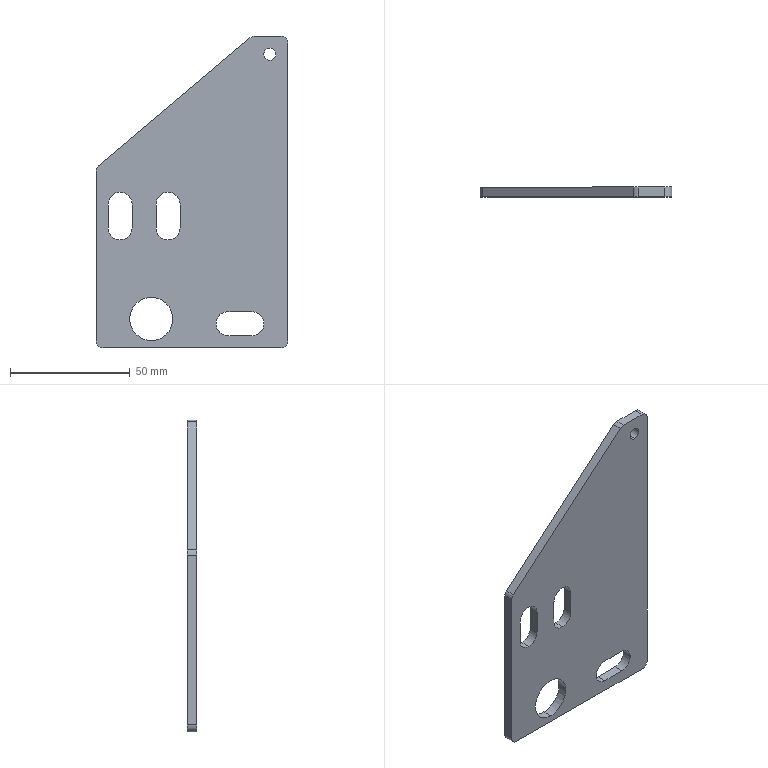Part | SolidWorks | features ExtruRefSurface 1, Extrusion 1, Fillet 1 | 1 solid | 30 faces | box 80 x 4 x 130 mm | volume 31186 mm3 | cylinder 17 | plane 13 | commonest cylinder face diameters 10 x8 6 x5 5 x2 18 x2
STEP:
#1=CARTESIAN_POINT('',(-7.5,4.,120.));
#2=VERTEX_POINT('',#1);
#3=CARTESIAN_POINT('',(-7.5,4.,125.));
#4=VERTEX_POINT('',#3);
#5=CARTESIAN_POINT('',(-7.5,4.,122.5));
#6=DIRECTION('',(0.,1.,0.));
#7=DIRECTION('',(0.,0.,1.));
#8=AXIS2_PLACEMENT_3D('',#5,#6,#7);
#9=CIRCLE('',#8,2.5);
#10=EDGE_CURVE('',#2,#4,#9,.T.);
#11=ORIENTED_EDGE('',*,*,#10,.T.);
#12=CARTESIAN_POINT('',(-7.5,0.,125.));
#13=VERTEX_POINT('',#12);
#14=CARTESIAN_POINT('',(-7.5,4.,125.));
#15=DIRECTION('',(0.,-1.,0.));
#16=VECTOR('',#15,1000.);
#17=LINE('',#14,#16);
#18=EDGE_CURVE('',#4,#13,#17,.T.);
#19=ORIENTED_EDGE('',*,*,#18,.T.);
#20=CARTESIAN_POINT('',(-7.5,0.,120.));
#21=VERTEX_POINT('',#20);
#22=CARTESIAN_POINT('',(-7.5,0.,122.5));
#23=DIRECTION('',(0.,1.,0.));
#24=DIRECTION('',(0.,0.,1.));
#25=AXIS2_PLACEMENT_3D('',#22,#23,#24);
#26=CIRCLE('',#25,2.5);
#27=EDGE_CURVE('',#21,#13,#26,.T.);
#28=ORIENTED_EDGE('',*,*,#27,.F.);
#29=CARTESIAN_POINT('',(-7.5,4.,120.));
#30=DIRECTION('',(0.,-1.,0.));
#31=VECTOR('',#30,1000.);
#32=LINE('',#29,#31);
#33=EDGE_CURVE('',#2,#21,#32,.T.);
#34=ORIENTED_EDGE('',*,*,#33,.F.);
#35=EDGE_LOOP('',(#11,#19,#28,#34));
#36=FACE_OUTER_BOUND('',#35,.T.);
#37=CARTESIAN_POINT('',(-7.5,4.,122.5));
#38=DIRECTION('',(0.,-1.,0.));
#39=DIRECTION('',(0.,0.,-1.));
#40=AXIS2_PLACEMENT_3D('',#37,#38,#39);
#41=CYLINDRICAL_SURFACE('',#40,2.5);
#42=ADVANCED_FACE('',(#36),#41,.F.);
#43=CARTESIAN_POINT('',(-45.,4.,50.));
#44=VERTEX_POINT('',#43);
#45=CARTESIAN_POINT('',(-50.,4.,45.));
#46=VERTEX_POINT('',#45);
#47=CARTESIAN_POINT('',(-50.,4.,50.));
#48=DIRECTION('',(0.,1.,0.));
#49=DIRECTION('',(0.,0.,1.));
#50=AXIS2_PLACEMENT_3D('',#47,#48,#49);
#51=CIRCLE('',#50,5.);
#52=EDGE_CURVE('',#44,#46,#51,.T.);
#53=ORIENTED_EDGE('',*,*,#52,.T.);
#54=CARTESIAN_POINT('',(-50.,0.,45.));
#55=VERTEX_POINT('',#54);
#56=CARTESIAN_POINT('',(-50.,4.,45.));
#57=DIRECTION('',(0.,-1.,0.));
#58=VECTOR('',#57,1000.);
#59=LINE('',#56,#58);
#60=EDGE_CURVE('',#46,#55,#59,.T.);
#61=ORIENTED_EDGE('',*,*,#60,.T.);
#62=CARTESIAN_POINT('',(-45.,0.,50.));
#63=VERTEX_POINT('',#62);
#64=CARTESIAN_POINT('',(-50.,0.,50.));
#65=DIRECTION('',(0.,1.,0.));
#66=DIRECTION('',(0.,0.,1.));
#67=AXIS2_PLACEMENT_3D('',#64,#65,#66);
#68=CIRCLE('',#67,5.);
#69=EDGE_CURVE('',#63,#55,#68,.T.);
#70=ORIENTED_EDGE('',*,*,#69,.F.);
#71=CARTESIAN_POINT('',(-45.,4.,50.));
#72=DIRECTION('',(0.,-1.,0.));
#73=VECTOR('',#72,1000.);
#74=LINE('',#71,#73);
#75=EDGE_CURVE('',#44,#63,#74,.T.);
#76=ORIENTED_EDGE('',*,*,#75,.F.);
#77=EDGE_LOOP('',(#53,#61,#70,#76));
#78=FACE_OUTER_BOUND('',#77,.T.);
#79=CARTESIAN_POINT('',(-50.,4.,50.));
#80=DIRECTION('',(0.,-1.,0.));
#81=DIRECTION('',(0.,0.,-1.));
#82=AXIS2_PLACEMENT_3D('',#79,#80,#81);
#83=CYLINDRICAL_SURFACE('',#82,5.);
#84=ADVANCED_FACE('',(#78),#83,.F.);
#85=CARTESIAN_POINT('',(-65.,4.,50.));
#86=VERTEX_POINT('',#85);
#87=CARTESIAN_POINT('',(-70.,4.,45.));
#88=VERTEX_POINT('',#87);
#89=CARTESIAN_POINT('',(-70.,4.,50.));
#90=DIRECTION('',(0.,1.,0.));
#91=DIRECTION('',(0.,0.,1.));
#92=AXIS2_PLACEMENT_3D('',#89,#90,#91);
#93=CIRCLE('',#92,5.);
#94=EDGE_CURVE('',#86,#88,#93,.T.);
#95=ORIENTED_EDGE('',*,*,#94,.T.);
#96=CARTESIAN_POINT('',(-70.,0.,45.));
#97=VERTEX_POINT('',#96);
#98=CARTESIAN_POINT('',(-70.,4.,45.));
#99=DIRECTION('',(0.,-1.,0.));
#100=VECTOR('',#99,1000.);
#101=LINE('',#98,#100);
#102=EDGE_CURVE('',#88,#97,#101,.T.);
#103=ORIENTED_EDGE('',*,*,#102,.T.);
#104=CARTESIAN_POINT('',(-65.,0.,50.));
#105=VERTEX_POINT('',#104);
#106=CARTESIAN_POINT('',(-70.,0.,50.));
#107=DIRECTION('',(0.,1.,0.));
#108=DIRECTION('',(0.,0.,1.));
#109=AXIS2_PLACEMENT_3D('',#106,#107,#108);
#110=CIRCLE('',#109,5.);
#111=EDGE_CURVE('',#105,#97,#110,.T.);
#112=ORIENTED_EDGE('',*,*,#111,.F.);
#113=CARTESIAN_POINT('',(-65.,4.,50.));
#114=DIRECTION('',(0.,-1.,0.));
#115=VECTOR('',#114,1000.);
#116=LINE('',#113,#115);
#117=EDGE_CURVE('',#86,#105,#116,.T.);
#118=ORIENTED_EDGE('',*,*,#117,.F.);
#119=EDGE_LOOP('',(#95,#103,#112,#118));
#120=FACE_OUTER_BOUND('',#119,.T.);
#121=CARTESIAN_POINT('',(-70.,4.,50.));
#122=DIRECTION('',(0.,-1.,0.));
#123=DIRECTION('',(0.,0.,-1.));
#124=AXIS2_PLACEMENT_3D('',#121,#122,#123);
#125=CYLINDRICAL_SURFACE('',#124,5.);
#126=ADVANCED_FACE('',(#120),#125,.F.);
#127=CARTESIAN_POINT('',(-57.,4.,3.));
#128=VERTEX_POINT('',#127);
#129=CARTESIAN_POINT('',(-57.,4.,21.));
#130=VERTEX_POINT('',#129);
#131=CARTESIAN_POINT('',(-57.,4.,12.));
#132=DIRECTION('',(0.,1.,0.));
#133=DIRECTION('',(0.,0.,1.));
#134=AXIS2_PLACEMENT_3D('',#131,#132,#133);
#135=CIRCLE('',#134,9.);
#136=EDGE_CURVE('',#128,#130,#135,.T.);
#137=ORIENTED_EDGE('',*,*,#136,.T.);
#138=CARTESIAN_POINT('',(-57.,0.,21.));
#139=VERTEX_POINT('',#138);
#140=CARTESIAN_POINT('',(-57.,4.,21.));
#141=DIRECTION('',(0.,-1.,0.));
#142=VECTOR('',#141,1000.);
#143=LINE('',#140,#142);
#144=EDGE_CURVE('',#130,#139,#143,.T.);
#145=ORIENTED_EDGE('',*,*,#144,.T.);
#146=CARTESIAN_POINT('',(-57.,0.,3.));
#147=VERTEX_POINT('',#146);
#148=CARTESIAN_POINT('',(-57.,0.,12.));
#149=DIRECTION('',(0.,1.,0.));
#150=DIRECTION('',(0.,0.,1.));
#151=AXIS2_PLACEMENT_3D('',#148,#149,#150);
#152=CIRCLE('',#151,9.);
#153=EDGE_CURVE('',#147,#139,#152,.T.);
#154=ORIENTED_EDGE('',*,*,#153,.F.);
#155=CARTESIAN_POINT('',(-57.,4.,3.));
#156=DIRECTION('',(0.,-1.,0.));
#157=VECTOR('',#156,1000.);
#158=LINE('',#155,#157);
#159=EDGE_CURVE('',#128,#147,#158,.T.);
#160=ORIENTED_EDGE('',*,*,#159,.F.);
#161=EDGE_LOOP('',(#137,#145,#154,#160));
#162=FACE_OUTER_BOUND('',#161,.T.);
#163=CARTESIAN_POINT('',(-57.,4.,12.));
#164=DIRECTION('',(0.,-1.,0.));
#165=DIRECTION('',(0.,0.,-1.));
#166=AXIS2_PLACEMENT_3D('',#163,#164,#165);
#167=CYLINDRICAL_SURFACE('',#166,9.);
#168=ADVANCED_FACE('',(#162),#167,.F.);
#169=CARTESIAN_POINT('',(-55.,4.,50.));
#170=VERTEX_POINT('',#169);
#171=CARTESIAN_POINT('',(-55.,4.,60.));
#172=VERTEX_POINT('',#171);
#173=CARTESIAN_POINT('',(-55.,4.,50.));
#174=DIRECTION('',(0.,0.,1.));
#175=VECTOR('',#174,1000.);
#176=LINE('',#173,#175);
#177=EDGE_CURVE('',#170,#172,#176,.T.);
#178=ORIENTED_EDGE('',*,*,#177,.F.);
#179=CARTESIAN_POINT('',(-50.,4.,50.));
#180=DIRECTION('',(0.,1.,0.));
#181=DIRECTION('',(0.,0.,1.));
#182=AXIS2_PLACEMENT_3D('',#179,#180,#181);
#183=CIRCLE('',#182,5.);
#184=EDGE_CURVE('',#46,#170,#183,.T.);
#185=ORIENTED_EDGE('',*,*,#184,.F.);
#186=ORIENTED_EDGE('',*,*,#52,.F.);
#187=CARTESIAN_POINT('',(-45.,4.,60.));
#188=VERTEX_POINT('',#187);
#189=CARTESIAN_POINT('',(-45.,4.,50.));
#190=DIRECTION('',(0.,0.,-1.));
#191=VECTOR('',#190,1000.);
#192=LINE('',#189,#191);
#193=EDGE_CURVE('',#188,#44,#192,.T.);
#194=ORIENTED_EDGE('',*,*,#193,.F.);
#195=CARTESIAN_POINT('',(-50.,4.,60.));
#196=DIRECTION('',(0.,1.,0.));
#197=DIRECTION('',(0.,0.,1.));
#198=AXIS2_PLACEMENT_3D('',#195,#196,#197);
#199=CIRCLE('',#198,5.);
#200=EDGE_CURVE('',#172,#188,#199,.T.);
#201=ORIENTED_EDGE('',*,*,#200,.F.);
#202=EDGE_LOOP('',(#178,#185,#186,#194,#201));
#203=FACE_BOUND('',#202,.T.);
#204=CARTESIAN_POINT('',(-75.,4.,50.));
#205=VERTEX_POINT('',#204);
#206=CARTESIAN_POINT('',(-75.,4.,60.));
#207=VERTEX_POINT('',#206);
#208=CARTESIAN_POINT('',(-75.,4.,50.));
#209=DIRECTION('',(0.,0.,1.));
#210=VECTOR('',#209,1000.);
#211=LINE('',#208,#210);
#212=EDGE_CURVE('',#205,#207,#211,.T.);
#213=ORIENTED_EDGE('',*,*,#212,.F.);
#214=CARTESIAN_POINT('',(-70.,4.,50.));
#215=DIRECTION('',(0.,1.,0.));
#216=DIRECTION('',(0.,0.,1.));
#217=AXIS2_PLACEMENT_3D('',#214,#215,#216);
#218=CIRCLE('',#217,5.);
#219=EDGE_CURVE('',#88,#205,#218,.T.);
#220=ORIENTED_EDGE('',*,*,#219,.F.);
#221=ORIENTED_EDGE('',*,*,#94,.F.);
#222=CARTESIAN_POINT('',(-65.,4.,60.));
#223=VERTEX_POINT('',#222);
#224=CARTESIAN_POINT('',(-65.,4.,50.));
#225=DIRECTION('',(0.,0.,-1.));
#226=VECTOR('',#225,1000.);
#227=LINE('',#224,#226);
#228=EDGE_CURVE('',#223,#86,#227,.T.);
#229=ORIENTED_EDGE('',*,*,#228,.F.);
#230=CARTESIAN_POINT('',(-70.,4.,60.));
#231=DIRECTION('',(0.,1.,0.));
#232=DIRECTION('',(0.,0.,1.));
#233=AXIS2_PLACEMENT_3D('',#230,#231,#232);
#234=CIRCLE('',#233,5.);
#235=EDGE_CURVE('',#207,#223,#234,.T.);
#236=ORIENTED_EDGE('',*,*,#235,.F.);
#237=EDGE_LOOP('',(#213,#220,#221,#229,#236));
#238=FACE_BOUND('',#237,.T.);
#239=CARTESIAN_POINT('',(-25.,4.,15.));
#240=VERTEX_POINT('',#239);
#241=CARTESIAN_POINT('',(-15.,4.,15.));
#242=VERTEX_POINT('',#241);
#243=CARTESIAN_POINT('',(-25.,4.,15.));
#244=DIRECTION('',(1.,0.,0.));
#245=VECTOR('',#244,1000.);
#246=LINE('',#243,#245);
#247=EDGE_CURVE('',#240,#242,#246,.T.);
#248=ORIENTED_EDGE('',*,*,#247,.F.);
#249=CARTESIAN_POINT('',(-25.,4.,5.));
#250=VERTEX_POINT('',#249);
#251=CARTESIAN_POINT('',(-25.,4.,10.));
#252=DIRECTION('',(0.,1.,0.));
#253=DIRECTION('',(0.,0.,1.));
#254=AXIS2_PLACEMENT_3D('',#251,#252,#253);
#255=CIRCLE('',#254,5.);
#256=EDGE_CURVE('',#250,#240,#255,.T.);
#257=ORIENTED_EDGE('',*,*,#256,.F.);
#258=CARTESIAN_POINT('',(-15.,4.,5.));
#259=VERTEX_POINT('',#258);
#260=CARTESIAN_POINT('',(-25.,4.,5.));
#261=DIRECTION('',(-1.,0.,0.));
#262=VECTOR('',#261,1000.);
#263=LINE('',#260,#262);
#264=EDGE_CURVE('',#259,#250,#263,.T.);
#265=ORIENTED_EDGE('',*,*,#264,.F.);
#266=CARTESIAN_POINT('',(-15.,4.,10.));
#267=DIRECTION('',(0.,1.,0.));
#268=DIRECTION('',(0.,0.,1.));
#269=AXIS2_PLACEMENT_3D('',#266,#267,#268);
#270=CIRCLE('',#269,5.);
#271=EDGE_CURVE('',#242,#259,#270,.T.);
#272=ORIENTED_EDGE('',*,*,#271,.F.);
#273=EDGE_LOOP('',(#248,#257,#265,#272));
#274=FACE_BOUND('',#273,.T.);
#275=ORIENTED_EDGE('',*,*,#136,.F.);
#276=CARTESIAN_POINT('',(-57.,4.,12.));
#277=DIRECTION('',(0.,1.,0.));
#278=DIRECTION('',(0.,0.,1.));
#279=AXIS2_PLACEMENT_3D('',#276,#277,#278);
#280=CIRCLE('',#279,9.);
#281=EDGE_CURVE('',#130,#128,#280,.T.);
#282=ORIENTED_EDGE('',*,*,#281,.F.);
#283=EDGE_LOOP('',(#275,#282));
#284=FACE_BOUND('',#283,.T.);
#285=CARTESIAN_POINT('',(-78.938,4.,75.899));
#286=VERTEX_POINT('',#285);
#287=CARTESIAN_POINT('',(-15.839,4.,129.29));
#288=VERTEX_POINT('',#287);
#289=CARTESIAN_POINT('',(-80.,4.,75.));
#290=DIRECTION('',(0.7634,0.,0.6459));
#291=VECTOR('',#290,1000.);
#292=LINE('',#289,#291);
#293=EDGE_CURVE('',#286,#288,#292,.T.);
#294=ORIENTED_EDGE('',*,*,#293,.T.);
#295=CARTESIAN_POINT('',(-13.901,4.,130.));
#296=VERTEX_POINT('',#295);
#297=CARTESIAN_POINT('',(-13.901,4.,127.));
#298=DIRECTION('',(0.,1.,0.));
#299=DIRECTION('',(0.,0.,1.));
#300=AXIS2_PLACEMENT_3D('',#297,#298,#299);
#301=CIRCLE('',#300,3.);
#302=EDGE_CURVE('',#288,#296,#301,.T.);
#303=ORIENTED_EDGE('',*,*,#302,.T.);
#304=CARTESIAN_POINT('',(-3.,4.,130.));
#305=VERTEX_POINT('',#304);
#306=CARTESIAN_POINT('',(-15.,4.,130.));
#307=DIRECTION('',(1.,0.,0.));
#308=VECTOR('',#307,1000.);
#309=LINE('',#306,#308);
#310=EDGE_CURVE('',#296,#305,#309,.T.);
#311=ORIENTED_EDGE('',*,*,#310,.T.);
#312=CARTESIAN_POINT('',(0.,4.,127.));
#313=VERTEX_POINT('',#312);
#314=CARTESIAN_POINT('',(-3.,4.,127.));
#315=DIRECTION('',(0.,1.,0.));
#316=DIRECTION('',(0.,0.,1.));
#317=AXIS2_PLACEMENT_3D('',#314,#315,#316);
#318=CIRCLE('',#317,3.);
#319=EDGE_CURVE('',#305,#313,#318,.T.);
#320=ORIENTED_EDGE('',*,*,#319,.T.);
#321=CARTESIAN_POINT('',(0.,4.,3.));
#322=VERTEX_POINT('',#321);
#323=CARTESIAN_POINT('',(0.,4.,130.));
#324=DIRECTION('',(0.,0.,-1.));
#325=VECTOR('',#324,1000.);
#326=LINE('',#323,#325);
#327=EDGE_CURVE('',#313,#322,#326,.T.);
#328=ORIENTED_EDGE('',*,*,#327,.T.);
#329=CARTESIAN_POINT('',(-3.,4.,0.));
#330=VERTEX_POINT('',#329);
#331=CARTESIAN_POINT('',(-3.,4.,3.));
#332=DIRECTION('',(0.,1.,0.));
#333=DIRECTION('',(0.,0.,1.));
#334=AXIS2_PLACEMENT_3D('',#331,#332,#333);
#335=CIRCLE('',#334,3.);
#336=EDGE_CURVE('',#322,#330,#335,.T.);
#337=ORIENTED_EDGE('',*,*,#336,.T.);
#338=CARTESIAN_POINT('',(-77.,4.,0.));
#339=VERTEX_POINT('',#338);
#340=CARTESIAN_POINT('',(0.,4.,0.));
#341=DIRECTION('',(-1.,0.,0.));
#342=VECTOR('',#341,1000.);
#343=LINE('',#340,#342);
#344=EDGE_CURVE('',#330,#339,#343,.T.);
#345=ORIENTED_EDGE('',*,*,#344,.T.);
#346=CARTESIAN_POINT('',(-80.,4.,3.));
#347=VERTEX_POINT('',#346);
#348=CARTESIAN_POINT('',(-77.,4.,3.));
#349=DIRECTION('',(0.,1.,0.));
#350=DIRECTION('',(0.,0.,1.));
#351=AXIS2_PLACEMENT_3D('',#348,#349,#350);
#352=CIRCLE('',#351,3.);
#353=EDGE_CURVE('',#339,#347,#352,.T.);
#354=ORIENTED_EDGE('',*,*,#353,.T.);
#355=CARTESIAN_POINT('',(-80.,4.,73.609));
#356=VERTEX_POINT('',#355);
#357=CARTESIAN_POINT('',(-80.,4.,0.));
#358=DIRECTION('',(0.,0.,1.));
#359=VECTOR('',#358,1000.);
#360=LINE('',#357,#359);
#361=EDGE_CURVE('',#347,#356,#360,.T.);
#362=ORIENTED_EDGE('',*,*,#361,.T.);
#363=CARTESIAN_POINT('',(-77.,4.,73.609));
#364=DIRECTION('',(0.,1.,0.));
#365=DIRECTION('',(0.,0.,1.));
#366=AXIS2_PLACEMENT_3D('',#363,#364,#365);
#367=CIRCLE('',#366,3.);
#368=EDGE_CURVE('',#356,#286,#367,.T.);
#369=ORIENTED_EDGE('',*,*,#368,.T.);
#370=EDGE_LOOP('',(#294,#303,#311,#320,#328,#337,#345,#354,#362,#369));
#371=FACE_OUTER_BOUND('',#370,.T.);
#372=ORIENTED_EDGE('',*,*,#10,.F.);
#373=CARTESIAN_POINT('',(-7.5,4.,122.5));
#374=DIRECTION('',(0.,1.,0.));
#375=DIRECTION('',(0.,0.,1.));
#376=AXIS2_PLACEMENT_3D('',#373,#374,#375);
#377=CIRCLE('',#376,2.5);
#378=EDGE_CURVE('',#4,#2,#377,.T.);
#379=ORIENTED_EDGE('',*,*,#378,.F.);
#380=EDGE_LOOP('',(#372,#379));
#381=FACE_BOUND('',#380,.T.);
#382=CARTESIAN_POINT('',(0.,4.,0.));
#383=DIRECTION('',(0.,1.,0.));
#384=DIRECTION('',(0.,0.,1.));
#385=AXIS2_PLACEMENT_3D('',#382,#383,#384);
#386=PLANE('',#385);
#387=ADVANCED_FACE('',(#203,#238,#274,#284,#371,#381),#386,.T.);
#388=ORIENTED_EDGE('',*,*,#111,.T.);
#389=CARTESIAN_POINT('',(-75.,0.,50.));
#390=VERTEX_POINT('',#389);
#391=CARTESIAN_POINT('',(-70.,0.,50.));
#392=DIRECTION('',(0.,1.,0.));
#393=DIRECTION('',(0.,0.,1.));
#394=AXIS2_PLACEMENT_3D('',#391,#392,#393);
#395=CIRCLE('',#394,5.);
#396=EDGE_CURVE('',#97,#390,#395,.T.);
#397=ORIENTED_EDGE('',*,*,#396,.T.);
#398=CARTESIAN_POINT('',(-75.,0.,60.));
#399=VERTEX_POINT('',#398);
#400=CARTESIAN_POINT('',(-75.,0.,50.));
#401=DIRECTION('',(0.,0.,1.));
#402=VECTOR('',#401,1000.);
#403=LINE('',#400,#402);
#404=EDGE_CURVE('',#390,#399,#403,.T.);
#405=ORIENTED_EDGE('',*,*,#404,.T.);
#406=CARTESIAN_POINT('',(-65.,0.,60.));
#407=VERTEX_POINT('',#406);
#408=CARTESIAN_POINT('',(-70.,0.,60.));
#409=DIRECTION('',(0.,1.,0.));
#410=DIRECTION('',(0.,0.,1.));
#411=AXIS2_PLACEMENT_3D('',#408,#409,#410);
#412=CIRCLE('',#411,5.);
#413=EDGE_CURVE('',#399,#407,#412,.T.);
#414=ORIENTED_EDGE('',*,*,#413,.T.);
#415=CARTESIAN_POINT('',(-65.,0.,50.));
#416=DIRECTION('',(0.,0.,-1.));
#417=VECTOR('',#416,1000.);
#418=LINE('',#415,#417);
#419=EDGE_CURVE('',#407,#105,#418,.T.);
#420=ORIENTED_EDGE('',*,*,#419,.T.);
#421=EDGE_LOOP('',(#388,#397,#405,#414,#420));
#422=FACE_BOUND('',#421,.T.);
#423=ORIENTED_EDGE('',*,*,#153,.T.);
#424=CARTESIAN_POINT('',(-57.,0.,12.));
#425=DIRECTION('',(0.,1.,0.));
#426=DIRECTION('',(0.,0.,1.));
#427=AXIS2_PLACEMENT_3D('',#424,#425,#426);
#428=CIRCLE('',#427,9.);
#429=EDGE_CURVE('',#139,#147,#428,.T.);
#430=ORIENTED_EDGE('',*,*,#429,.T.);
#431=EDGE_LOOP('',(#423,#430));
#432=FACE_BOUND('',#431,.T.);
#433=CARTESIAN_POINT('',(-13.901,0.,130.));
#434=VERTEX_POINT('',#433);
#435=CARTESIAN_POINT('',(-3.,0.,130.));
#436=VERTEX_POINT('',#435);
#437=CARTESIAN_POINT('',(-15.,0.,130.));
#438=DIRECTION('',(1.,0.,0.));
#439=VECTOR('',#438,1000.);
#440=LINE('',#437,#439);
#441=EDGE_CURVE('',#434,#436,#440,.T.);
#442=ORIENTED_EDGE('',*,*,#441,.F.);
#443=CARTESIAN_POINT('',(-15.839,0.,129.29));
#444=VERTEX_POINT('',#443);
#445=CARTESIAN_POINT('',(-13.901,0.,127.));
#446=DIRECTION('',(0.,-1.,0.));
#447=DIRECTION('',(0.,0.,1.));
#448=AXIS2_PLACEMENT_3D('',#445,#446,#447);
#449=CIRCLE('',#448,3.);
#450=EDGE_CURVE('',#434,#444,#449,.T.);
#451=ORIENTED_EDGE('',*,*,#450,.T.);
#452=CARTESIAN_POINT('',(-78.938,0.,75.899));
#453=VERTEX_POINT('',#452);
#454=CARTESIAN_POINT('',(-80.,0.,75.));
#455=DIRECTION('',(0.7634,0.,0.6459));
#456=VECTOR('',#455,1000.);
#457=LINE('',#454,#456);
#458=EDGE_CURVE('',#453,#444,#457,.T.);
#459=ORIENTED_EDGE('',*,*,#458,.F.);
#460=CARTESIAN_POINT('',(-80.,0.,73.609));
#461=VERTEX_POINT('',#460);
#462=CARTESIAN_POINT('',(-77.,0.,73.609));
#463=DIRECTION('',(0.,-1.,0.));
#464=DIRECTION('',(0.,0.,1.));
#465=AXIS2_PLACEMENT_3D('',#462,#463,#464);
#466=CIRCLE('',#465,3.);
#467=EDGE_CURVE('',#453,#461,#466,.T.);
#468=ORIENTED_EDGE('',*,*,#467,.T.);
#469=CARTESIAN_POINT('',(-80.,0.,3.));
#470=VERTEX_POINT('',#469);
#471=CARTESIAN_POINT('',(-80.,0.,0.));
#472=DIRECTION('',(0.,0.,1.));
#473=VECTOR('',#472,1000.);
#474=LINE('',#471,#473);
#475=EDGE_CURVE('',#470,#461,#474,.T.);
#476=ORIENTED_EDGE('',*,*,#475,.F.);
#477=CARTESIAN_POINT('',(-77.,0.,0.));
#478=VERTEX_POINT('',#477);
#479=CARTESIAN_POINT('',(-77.,0.,3.));
#480=DIRECTION('',(0.,-1.,0.));
#481=DIRECTION('',(0.,0.,1.));
#482=AXIS2_PLACEMENT_3D('',#479,#480,#481);
#483=CIRCLE('',#482,3.);
#484=EDGE_CURVE('',#470,#478,#483,.T.);
#485=ORIENTED_EDGE('',*,*,#484,.T.);
#486=CARTESIAN_POINT('',(-3.,0.,0.));
#487=VERTEX_POINT('',#486);
#488=CARTESIAN_POINT('',(0.,0.,0.));
#489=DIRECTION('',(-1.,0.,0.));
#490=VECTOR('',#489,1000.);
#491=LINE('',#488,#490);
#492=EDGE_CURVE('',#487,#478,#491,.T.);
#493=ORIENTED_EDGE('',*,*,#492,.F.);
#494=CARTESIAN_POINT('',(0.,0.,3.));
#495=VERTEX_POINT('',#494);
#496=CARTESIAN_POINT('',(-3.,0.,3.));
#497=DIRECTION('',(0.,-1.,0.));
#498=DIRECTION('',(0.,0.,1.));
#499=AXIS2_PLACEMENT_3D('',#496,#497,#498);
#500=CIRCLE('',#499,3.);
#501=EDGE_CURVE('',#487,#495,#500,.T.);
#502=ORIENTED_EDGE('',*,*,#501,.T.);
#503=CARTESIAN_POINT('',(0.,0.,127.));
#504=VERTEX_POINT('',#503);
#505=CARTESIAN_POINT('',(0.,0.,130.));
#506=DIRECTION('',(0.,0.,-1.));
#507=VECTOR('',#506,1000.);
#508=LINE('',#505,#507);
#509=EDGE_CURVE('',#504,#495,#508,.T.);
#510=ORIENTED_EDGE('',*,*,#509,.F.);
#511=CARTESIAN_POINT('',(-3.,0.,127.));
#512=DIRECTION('',(0.,-1.,0.));
#513=DIRECTION('',(0.,0.,1.));
#514=AXIS2_PLACEMENT_3D('',#511,#512,#513);
#515=CIRCLE('',#514,3.);
#516=EDGE_CURVE('',#504,#436,#515,.T.);
#517=ORIENTED_EDGE('',*,*,#516,.T.);
#518=EDGE_LOOP('',(#442,#451,#459,#468,#476,#485,#493,#502,#510,#517));
#519=FACE_OUTER_BOUND('',#518,.T.);
#520=CARTESIAN_POINT('',(-25.,0.,5.));
#521=VERTEX_POINT('',#520);
#522=CARTESIAN_POINT('',(-25.,0.,15.));
#523=VERTEX_POINT('',#522);
#524=CARTESIAN_POINT('',(-25.,0.,10.));
#525=DIRECTION('',(0.,1.,0.));
#526=DIRECTION('',(0.,0.,1.));
#527=AXIS2_PLACEMENT_3D('',#524,#525,#526);
#528=CIRCLE('',#527,5.);
#529=EDGE_CURVE('',#521,#523,#528,.T.);
#530=ORIENTED_EDGE('',*,*,#529,.T.);
#531=CARTESIAN_POINT('',(-15.,0.,15.));
#532=VERTEX_POINT('',#531);
#533=CARTESIAN_POINT('',(-25.,0.,15.));
#534=DIRECTION('',(1.,0.,0.));
#535=VECTOR('',#534,1000.);
#536=LINE('',#533,#535);
#537=EDGE_CURVE('',#523,#532,#536,.T.);
#538=ORIENTED_EDGE('',*,*,#537,.T.);
#539=CARTESIAN_POINT('',(-15.,0.,5.));
#540=VERTEX_POINT('',#539);
#541=CARTESIAN_POINT('',(-15.,0.,10.));
#542=DIRECTION('',(0.,1.,0.));
#543=DIRECTION('',(0.,0.,1.));
#544=AXIS2_PLACEMENT_3D('',#541,#542,#543);
#545=CIRCLE('',#544,5.);
#546=EDGE_CURVE('',#532,#540,#545,.T.);
#547=ORIENTED_EDGE('',*,*,#546,.T.);
#548=CARTESIAN_POINT('',(-25.,0.,5.));
#549=DIRECTION('',(-1.,0.,0.));
#550=VECTOR('',#549,1000.);
#551=LINE('',#548,#550);
#552=EDGE_CURVE('',#540,#521,#551,.T.);
#553=ORIENTED_EDGE('',*,*,#552,.T.);
#554=EDGE_LOOP('',(#530,#538,#547,#553));
#555=FACE_BOUND('',#554,.T.);
#556=ORIENTED_EDGE('',*,*,#69,.T.);
#557=CARTESIAN_POINT('',(-55.,0.,50.));
#558=VERTEX_POINT('',#557);
#559=CARTESIAN_POINT('',(-50.,0.,50.));
#560=DIRECTION('',(0.,1.,0.));
#561=DIRECTION('',(0.,0.,1.));
#562=AXIS2_PLACEMENT_3D('',#559,#560,#561);
#563=CIRCLE('',#562,5.);
#564=EDGE_CURVE('',#55,#558,#563,.T.);
#565=ORIENTED_EDGE('',*,*,#564,.T.);
#566=CARTESIAN_POINT('',(-55.,0.,60.));
#567=VERTEX_POINT('',#566);
#568=CARTESIAN_POINT('',(-55.,0.,50.));
#569=DIRECTION('',(0.,0.,1.));
#570=VECTOR('',#569,1000.);
#571=LINE('',#568,#570);
#572=EDGE_CURVE('',#558,#567,#571,.T.);
#573=ORIENTED_EDGE('',*,*,#572,.T.);
#574=CARTESIAN_POINT('',(-45.,0.,60.));
#575=VERTEX_POINT('',#574);
#576=CARTESIAN_POINT('',(-50.,0.,60.));
#577=DIRECTION('',(0.,1.,0.));
#578=DIRECTION('',(0.,0.,1.));
#579=AXIS2_PLACEMENT_3D('',#576,#577,#578);
#580=CIRCLE('',#579,5.);
#581=EDGE_CURVE('',#567,#575,#580,.T.);
#582=ORIENTED_EDGE('',*,*,#581,.T.);
#583=CARTESIAN_POINT('',(-45.,0.,50.));
#584=DIRECTION('',(0.,0.,-1.));
#585=VECTOR('',#584,1000.);
#586=LINE('',#583,#585);
#587=EDGE_CURVE('',#575,#63,#586,.T.);
#588=ORIENTED_EDGE('',*,*,#587,.T.);
#589=EDGE_LOOP('',(#556,#565,#573,#582,#588));
#590=FACE_BOUND('',#589,.T.);
#591=ORIENTED_EDGE('',*,*,#27,.T.);
#592=CARTESIAN_POINT('',(-7.5,0.,122.5));
#593=DIRECTION('',(0.,1.,0.));
#594=DIRECTION('',(0.,0.,1.));
#595=AXIS2_PLACEMENT_3D('',#592,#593,#594);
#596=CIRCLE('',#595,2.5);
#597=EDGE_CURVE('',#13,#21,#596,.T.);
#598=ORIENTED_EDGE('',*,*,#597,.T.);
#599=EDGE_LOOP('',(#591,#598));
#600=FACE_BOUND('',#599,.T.);
#601=CARTESIAN_POINT('',(0.,0.,0.));
#602=DIRECTION('',(0.,1.,0.));
#603=DIRECTION('',(0.,0.,1.));
#604=AXIS2_PLACEMENT_3D('',#601,#602,#603);
#605=PLANE('',#604);
#606=ADVANCED_FACE('',(#422,#432,#519,#555,#590,#600),#605,.F.);
#607=ORIENTED_EDGE('',*,*,#509,.T.);
#608=CARTESIAN_POINT('',(0.,4.,3.));
#609=DIRECTION('',(0.,1.,0.));
#610=VECTOR('',#609,1000.);
#611=LINE('',#608,#610);
#612=EDGE_CURVE('',#495,#322,#611,.T.);
#613=ORIENTED_EDGE('',*,*,#612,.T.);
#614=ORIENTED_EDGE('',*,*,#327,.F.);
#615=CARTESIAN_POINT('',(0.,4.,127.));
#616=DIRECTION('',(0.,-1.,0.));
#617=VECTOR('',#616,1000.);
#618=LINE('',#615,#617);
#619=EDGE_CURVE('',#313,#504,#618,.T.);
#620=ORIENTED_EDGE('',*,*,#619,.T.);
#621=EDGE_LOOP('',(#607,#613,#614,#620));
#622=FACE_OUTER_BOUND('',#621,.T.);
#623=CARTESIAN_POINT('',(0.,4.,130.));
#624=DIRECTION('',(-1.,0.,0.));
#625=DIRECTION('',(0.,0.,1.));
#626=AXIS2_PLACEMENT_3D('',#623,#624,#625);
#627=PLANE('',#626);
#628=ADVANCED_FACE('',(#622),#627,.F.);
#629=ORIENTED_EDGE('',*,*,#492,.T.);
#630=CARTESIAN_POINT('',(-77.,4.,0.));
#631=DIRECTION('',(0.,1.,0.));
#632=VECTOR('',#631,1000.);
#633=LINE('',#630,#632);
#634=EDGE_CURVE('',#478,#339,#633,.T.);
#635=ORIENTED_EDGE('',*,*,#634,.T.);
#636=ORIENTED_EDGE('',*,*,#344,.F.);
#637=CARTESIAN_POINT('',(-3.,4.,0.));
#638=DIRECTION('',(0.,-1.,0.));
#639=VECTOR('',#638,1000.);
#640=LINE('',#637,#639);
#641=EDGE_CURVE('',#330,#487,#640,.T.);
#642=ORIENTED_EDGE('',*,*,#641,.T.);
#643=EDGE_LOOP('',(#629,#635,#636,#642));
#644=FACE_OUTER_BOUND('',#643,.T.);
#645=CARTESIAN_POINT('',(0.,4.,0.));
#646=DIRECTION('',(0.,0.,1.));
#647=DIRECTION('',(1.,0.,0.));
#648=AXIS2_PLACEMENT_3D('',#645,#646,#647);
#649=PLANE('',#648);
#650=ADVANCED_FACE('',(#644),#649,.F.);
#651=ORIENTED_EDGE('',*,*,#475,.T.);
#652=CARTESIAN_POINT('',(-80.,4.,73.609));
#653=DIRECTION('',(0.,1.,0.));
#654=VECTOR('',#653,1000.);
#655=LINE('',#652,#654);
#656=EDGE_CURVE('',#461,#356,#655,.T.);
#657=ORIENTED_EDGE('',*,*,#656,.T.);
#658=ORIENTED_EDGE('',*,*,#361,.F.);
#659=CARTESIAN_POINT('',(-80.,4.,3.));
#660=DIRECTION('',(0.,-1.,0.));
#661=VECTOR('',#660,1000.);
#662=LINE('',#659,#661);
#663=EDGE_CURVE('',#347,#470,#662,.T.);
#664=ORIENTED_EDGE('',*,*,#663,.T.);
#665=EDGE_LOOP('',(#651,#657,#658,#664));
#666=FACE_OUTER_BOUND('',#665,.T.);
#667=CARTESIAN_POINT('',(-80.,4.,0.));
#668=DIRECTION('',(1.,0.,0.));
#669=DIRECTION('',(0.,0.,-1.));
#670=AXIS2_PLACEMENT_3D('',#667,#668,#669);
#671=PLANE('',#670);
#672=ADVANCED_FACE('',(#666),#671,.F.);
#673=ORIENTED_EDGE('',*,*,#458,.T.);
#674=CARTESIAN_POINT('',(-15.839,4.,129.29));
#675=DIRECTION('',(0.,1.,0.));
#676=VECTOR('',#675,1000.);
#677=LINE('',#674,#676);
#678=EDGE_CURVE('',#444,#288,#677,.T.);
#679=ORIENTED_EDGE('',*,*,#678,.T.);
#680=ORIENTED_EDGE('',*,*,#293,.F.);
#681=CARTESIAN_POINT('',(-78.938,4.,75.899));
#682=DIRECTION('',(0.,-1.,0.));
#683=VECTOR('',#682,1000.);
#684=LINE('',#681,#683);
#685=EDGE_CURVE('',#286,#453,#684,.T.);
#686=ORIENTED_EDGE('',*,*,#685,.T.);
#687=EDGE_LOOP('',(#673,#679,#680,#686));
#688=FACE_OUTER_BOUND('',#687,.T.);
#689=CARTESIAN_POINT('',(-80.,4.,75.));
#690=DIRECTION('',(0.6459,0.,-0.7634));
#691=DIRECTION('',(-0.7634,0.,-0.6459));
#692=AXIS2_PLACEMENT_3D('',#689,#690,#691);
#693=PLANE('',#692);
#694=ADVANCED_FACE('',(#688),#693,.F.);
#695=ORIENTED_EDGE('',*,*,#310,.F.);
#696=CARTESIAN_POINT('',(-13.901,4.,130.));
#697=DIRECTION('',(0.,-1.,0.));
#698=VECTOR('',#697,1000.);
#699=LINE('',#696,#698);
#700=EDGE_CURVE('',#296,#434,#699,.T.);
#701=ORIENTED_EDGE('',*,*,#700,.T.);
#702=ORIENTED_EDGE('',*,*,#441,.T.);
#703=CARTESIAN_POINT('',(-3.,4.,130.));
#704=DIRECTION('',(0.,1.,0.));
#705=VECTOR('',#704,1000.);
#706=LINE('',#703,#705);
#707=EDGE_CURVE('',#436,#305,#706,.T.);
#708=ORIENTED_EDGE('',*,*,#707,.T.);
#709=EDGE_LOOP('',(#695,#701,#702,#708));
#710=FACE_OUTER_BOUND('',#709,.T.);
#711=CARTESIAN_POINT('',(-15.,4.,130.));
#712=DIRECTION('',(0.,0.,-1.));
#713=DIRECTION('',(-1.,0.,0.));
#714=AXIS2_PLACEMENT_3D('',#711,#712,#713);
#715=PLANE('',#714);
#716=ADVANCED_FACE('',(#710),#715,.F.);
#717=ORIENTED_EDGE('',*,*,#144,.F.);
#718=ORIENTED_EDGE('',*,*,#281,.T.);
#719=ORIENTED_EDGE('',*,*,#159,.T.);
#720=ORIENTED_EDGE('',*,*,#429,.F.);
#721=EDGE_LOOP('',(#717,#718,#719,#720));
#722=FACE_OUTER_BOUND('',#721,.T.);
#723=CARTESIAN_POINT('',(-57.,4.,12.));
#724=DIRECTION('',(0.,-1.,0.));
#725=DIRECTION('',(0.,0.,-1.));
#726=AXIS2_PLACEMENT_3D('',#723,#724,#725);
#727=CYLINDRICAL_SURFACE('',#726,9.);
#728=ADVANCED_FACE('',(#722),#727,.F.);
#729=ORIENTED_EDGE('',*,*,#529,.F.);
#730=CARTESIAN_POINT('',(-25.,4.,5.));
#731=DIRECTION('',(0.,-1.,0.));
#732=VECTOR('',#731,1000.);
#733=LINE('',#730,#732);
#734=EDGE_CURVE('',#250,#521,#733,.T.);
#735=ORIENTED_EDGE('',*,*,#734,.F.);
#736=ORIENTED_EDGE('',*,*,#256,.T.);
#737=CARTESIAN_POINT('',(-25.,4.,15.));
#738=DIRECTION('',(0.,-1.,0.));
#739=VECTOR('',#738,1000.);
#740=LINE('',#737,#739);
#741=EDGE_CURVE('',#240,#523,#740,.T.);
#742=ORIENTED_EDGE('',*,*,#741,.T.);
#743=EDGE_LOOP('',(#729,#735,#736,#742));
#744=FACE_OUTER_BOUND('',#743,.T.);
#745=CARTESIAN_POINT('',(-25.,4.,10.));
#746=DIRECTION('',(0.,-1.,0.));
#747=DIRECTION('',(0.,0.,-1.));
#748=AXIS2_PLACEMENT_3D('',#745,#746,#747);
#749=CYLINDRICAL_SURFACE('',#748,5.);
#750=ADVANCED_FACE('',(#744),#749,.F.);
#751=ORIENTED_EDGE('',*,*,#537,.F.);
#752=ORIENTED_EDGE('',*,*,#741,.F.);
#753=ORIENTED_EDGE('',*,*,#247,.T.);
#754=CARTESIAN_POINT('',(-15.,4.,15.));
#755=DIRECTION('',(0.,-1.,0.));
#756=VECTOR('',#755,1000.);
#757=LINE('',#754,#756);
#758=EDGE_CURVE('',#242,#532,#757,.T.);
#759=ORIENTED_EDGE('',*,*,#758,.T.);
#760=EDGE_LOOP('',(#751,#752,#753,#759));
#761=FACE_OUTER_BOUND('',#760,.T.);
#762=CARTESIAN_POINT('',(-25.,4.,15.));
#763=DIRECTION('',(0.,0.,-1.));
#764=DIRECTION('',(-1.,0.,0.));
#765=AXIS2_PLACEMENT_3D('',#762,#763,#764);
#766=PLANE('',#765);
#767=ADVANCED_FACE('',(#761),#766,.T.);
#768=ORIENTED_EDGE('',*,*,#546,.F.);
#769=ORIENTED_EDGE('',*,*,#758,.F.);
#770=ORIENTED_EDGE('',*,*,#271,.T.);
#771=CARTESIAN_POINT('',(-15.,4.,5.));
#772=DIRECTION('',(0.,-1.,0.));
#773=VECTOR('',#772,1000.);
#774=LINE('',#771,#773);
#775=EDGE_CURVE('',#259,#540,#774,.T.);
#776=ORIENTED_EDGE('',*,*,#775,.T.);
#777=EDGE_LOOP('',(#768,#769,#770,#776));
#778=FACE_OUTER_BOUND('',#777,.T.);
#779=CARTESIAN_POINT('',(-15.,4.,10.));
#780=DIRECTION('',(0.,-1.,0.));
#781=DIRECTION('',(0.,0.,-1.));
#782=AXIS2_PLACEMENT_3D('',#779,#780,#781);
#783=CYLINDRICAL_SURFACE('',#782,5.);
#784=ADVANCED_FACE('',(#778),#783,.F.);
#785=ORIENTED_EDGE('',*,*,#552,.F.);
#786=ORIENTED_EDGE('',*,*,#775,.F.);
#787=ORIENTED_EDGE('',*,*,#264,.T.);
#788=ORIENTED_EDGE('',*,*,#734,.T.);
#789=EDGE_LOOP('',(#785,#786,#787,#788));
#790=FACE_OUTER_BOUND('',#789,.T.);
#791=CARTESIAN_POINT('',(-25.,4.,5.));
#792=DIRECTION('',(0.,0.,1.));
#793=DIRECTION('',(1.,0.,0.));
#794=AXIS2_PLACEMENT_3D('',#791,#792,#793);
#795=PLANE('',#794);
#796=ADVANCED_FACE('',(#790),#795,.T.);
#797=ORIENTED_EDGE('',*,*,#102,.F.);
#798=ORIENTED_EDGE('',*,*,#219,.T.);
#799=CARTESIAN_POINT('',(-75.,4.,50.));
#800=DIRECTION('',(0.,-1.,0.));
#801=VECTOR('',#800,1000.);
#802=LINE('',#799,#801);
#803=EDGE_CURVE('',#205,#390,#802,.T.);
#804=ORIENTED_EDGE('',*,*,#803,.T.);
#805=ORIENTED_EDGE('',*,*,#396,.F.);
#806=EDGE_LOOP('',(#797,#798,#804,#805));
#807=FACE_OUTER_BOUND('',#806,.T.);
#808=CARTESIAN_POINT('',(-70.,4.,50.));
#809=DIRECTION('',(0.,-1.,0.));
#810=DIRECTION('',(0.,0.,-1.));
#811=AXIS2_PLACEMENT_3D('',#808,#809,#810);
#812=CYLINDRICAL_SURFACE('',#811,5.);
#813=ADVANCED_FACE('',(#807),#812,.F.);
#814=ORIENTED_EDGE('',*,*,#404,.F.);
#815=ORIENTED_EDGE('',*,*,#803,.F.);
#816=ORIENTED_EDGE('',*,*,#212,.T.);
#817=CARTESIAN_POINT('',(-75.,4.,60.));
#818=DIRECTION('',(0.,-1.,0.));
#819=VECTOR('',#818,1000.);
#820=LINE('',#817,#819);
#821=EDGE_CURVE('',#207,#399,#820,.T.);
#822=ORIENTED_EDGE('',*,*,#821,.T.);
#823=EDGE_LOOP('',(#814,#815,#816,#822));
#824=FACE_OUTER_BOUND('',#823,.T.);
#825=CARTESIAN_POINT('',(-75.,4.,50.));
#826=DIRECTION('',(1.,0.,0.));
#827=DIRECTION('',(0.,0.,-1.));
#828=AXIS2_PLACEMENT_3D('',#825,#826,#827);
#829=PLANE('',#828);
#830=ADVANCED_FACE('',(#824),#829,.T.);
#831=ORIENTED_EDGE('',*,*,#413,.F.);
#832=ORIENTED_EDGE('',*,*,#821,.F.);
#833=ORIENTED_EDGE('',*,*,#235,.T.);
#834=CARTESIAN_POINT('',(-65.,4.,60.));
#835=DIRECTION('',(0.,-1.,0.));
#836=VECTOR('',#835,1000.);
#837=LINE('',#834,#836);
#838=EDGE_CURVE('',#223,#407,#837,.T.);
#839=ORIENTED_EDGE('',*,*,#838,.T.);
#840=EDGE_LOOP('',(#831,#832,#833,#839));
#841=FACE_OUTER_BOUND('',#840,.T.);
#842=CARTESIAN_POINT('',(-70.,4.,60.));
#843=DIRECTION('',(0.,-1.,0.));
#844=DIRECTION('',(0.,0.,-1.));
#845=AXIS2_PLACEMENT_3D('',#842,#843,#844);
#846=CYLINDRICAL_SURFACE('',#845,5.);
#847=ADVANCED_FACE('',(#841),#846,.F.);
#848=ORIENTED_EDGE('',*,*,#419,.F.);
#849=ORIENTED_EDGE('',*,*,#838,.F.);
#850=ORIENTED_EDGE('',*,*,#228,.T.);
#851=ORIENTED_EDGE('',*,*,#117,.T.);
#852=EDGE_LOOP('',(#848,#849,#850,#851));
#853=FACE_OUTER_BOUND('',#852,.T.);
#854=CARTESIAN_POINT('',(-65.,4.,50.));
#855=DIRECTION('',(-1.,0.,0.));
#856=DIRECTION('',(0.,0.,1.));
#857=AXIS2_PLACEMENT_3D('',#854,#855,#856);
#858=PLANE('',#857);
#859=ADVANCED_FACE('',(#853),#858,.T.);
#860=ORIENTED_EDGE('',*,*,#60,.F.);
#861=ORIENTED_EDGE('',*,*,#184,.T.);
#862=CARTESIAN_POINT('',(-55.,4.,50.));
#863=DIRECTION('',(0.,-1.,0.));
#864=VECTOR('',#863,1000.);
#865=LINE('',#862,#864);
#866=EDGE_CURVE('',#170,#558,#865,.T.);
#867=ORIENTED_EDGE('',*,*,#866,.T.);
#868=ORIENTED_EDGE('',*,*,#564,.F.);
#869=EDGE_LOOP('',(#860,#861,#867,#868));
#870=FACE_OUTER_BOUND('',#869,.T.);
#871=CARTESIAN_POINT('',(-50.,4.,50.));
#872=DIRECTION('',(0.,-1.,0.));
#873=DIRECTION('',(0.,0.,-1.));
#874=AXIS2_PLACEMENT_3D('',#871,#872,#873);
#875=CYLINDRICAL_SURFACE('',#874,5.);
#876=ADVANCED_FACE('',(#870),#875,.F.);
#877=ORIENTED_EDGE('',*,*,#572,.F.);
#878=ORIENTED_EDGE('',*,*,#866,.F.);
#879=ORIENTED_EDGE('',*,*,#177,.T.);
#880=CARTESIAN_POINT('',(-55.,4.,60.));
#881=DIRECTION('',(0.,-1.,0.));
#882=VECTOR('',#881,1000.);
#883=LINE('',#880,#882);
#884=EDGE_CURVE('',#172,#567,#883,.T.);
#885=ORIENTED_EDGE('',*,*,#884,.T.);
#886=EDGE_LOOP('',(#877,#878,#879,#885));
#887=FACE_OUTER_BOUND('',#886,.T.);
#888=CARTESIAN_POINT('',(-55.,4.,50.));
#889=DIRECTION('',(1.,0.,0.));
#890=DIRECTION('',(0.,0.,-1.));
#891=AXIS2_PLACEMENT_3D('',#888,#889,#890);
#892=PLANE('',#891);
#893=ADVANCED_FACE('',(#887),#892,.T.);
#894=ORIENTED_EDGE('',*,*,#581,.F.);
#895=ORIENTED_EDGE('',*,*,#884,.F.);
#896=ORIENTED_EDGE('',*,*,#200,.T.);
#897=CARTESIAN_POINT('',(-45.,4.,60.));
#898=DIRECTION('',(0.,-1.,0.));
#899=VECTOR('',#898,1000.);
#900=LINE('',#897,#899);
#901=EDGE_CURVE('',#188,#575,#900,.T.);
#902=ORIENTED_EDGE('',*,*,#901,.T.);
#903=EDGE_LOOP('',(#894,#895,#896,#902));
#904=FACE_OUTER_BOUND('',#903,.T.);
#905=CARTESIAN_POINT('',(-50.,4.,60.));
#906=DIRECTION('',(0.,-1.,0.));
#907=DIRECTION('',(0.,0.,-1.));
#908=AXIS2_PLACEMENT_3D('',#905,#906,#907);
#909=CYLINDRICAL_SURFACE('',#908,5.);
#910=ADVANCED_FACE('',(#904),#909,.F.);
#911=ORIENTED_EDGE('',*,*,#587,.F.);
#912=ORIENTED_EDGE('',*,*,#901,.F.);
#913=ORIENTED_EDGE('',*,*,#193,.T.);
#914=ORIENTED_EDGE('',*,*,#75,.T.);
#915=EDGE_LOOP('',(#911,#912,#913,#914));
#916=FACE_OUTER_BOUND('',#915,.T.);
#917=CARTESIAN_POINT('',(-45.,4.,50.));
#918=DIRECTION('',(-1.,0.,0.));
#919=DIRECTION('',(0.,0.,1.));
#920=AXIS2_PLACEMENT_3D('',#917,#918,#919);
#921=PLANE('',#920);
#922=ADVANCED_FACE('',(#916),#921,.T.);
#923=ORIENTED_EDGE('',*,*,#18,.F.);
#924=ORIENTED_EDGE('',*,*,#378,.T.);
#925=ORIENTED_EDGE('',*,*,#33,.T.);
#926=ORIENTED_EDGE('',*,*,#597,.F.);
#927=EDGE_LOOP('',(#923,#924,#925,#926));
#928=FACE_OUTER_BOUND('',#927,.T.);
#929=CARTESIAN_POINT('',(-7.5,4.,122.5));
#930=DIRECTION('',(0.,-1.,0.));
#931=DIRECTION('',(0.,0.,-1.));
#932=AXIS2_PLACEMENT_3D('',#929,#930,#931);
#933=CYLINDRICAL_SURFACE('',#932,2.5);
#934=ADVANCED_FACE('',(#928),#933,.F.);
#935=ORIENTED_EDGE('',*,*,#302,.F.);
#936=ORIENTED_EDGE('',*,*,#678,.F.);
#937=ORIENTED_EDGE('',*,*,#450,.F.);
#938=ORIENTED_EDGE('',*,*,#700,.F.);
#939=EDGE_LOOP('',(#935,#936,#937,#938));
#940=FACE_OUTER_BOUND('',#939,.T.);
#941=CARTESIAN_POINT('',(-13.901,4.,127.));
#942=DIRECTION('',(0.,-1.,0.));
#943=DIRECTION('',(0.,0.,-1.));
#944=AXIS2_PLACEMENT_3D('',#941,#942,#943);
#945=CYLINDRICAL_SURFACE('',#944,3.);
#946=ADVANCED_FACE('',(#940),#945,.T.);
#947=ORIENTED_EDGE('',*,*,#368,.F.);
#948=ORIENTED_EDGE('',*,*,#656,.F.);
#949=ORIENTED_EDGE('',*,*,#467,.F.);
#950=ORIENTED_EDGE('',*,*,#685,.F.);
#951=EDGE_LOOP('',(#947,#948,#949,#950));
#952=FACE_OUTER_BOUND('',#951,.T.);
#953=CARTESIAN_POINT('',(-77.,4.,73.609));
#954=DIRECTION('',(0.,-1.,0.));
#955=DIRECTION('',(0.,0.,-1.));
#956=AXIS2_PLACEMENT_3D('',#953,#954,#955);
#957=CYLINDRICAL_SURFACE('',#956,3.);
#958=ADVANCED_FACE('',(#952),#957,.T.);
#959=ORIENTED_EDGE('',*,*,#353,.F.);
#960=ORIENTED_EDGE('',*,*,#634,.F.);
#961=ORIENTED_EDGE('',*,*,#484,.F.);
#962=ORIENTED_EDGE('',*,*,#663,.F.);
#963=EDGE_LOOP('',(#959,#960,#961,#962));
#964=FACE_OUTER_BOUND('',#963,.T.);
#965=CARTESIAN_POINT('',(-77.,4.,3.));
#966=DIRECTION('',(0.,-1.,0.));
#967=DIRECTION('',(0.,0.,-1.));
#968=AXIS2_PLACEMENT_3D('',#965,#966,#967);
#969=CYLINDRICAL_SURFACE('',#968,3.);
#970=ADVANCED_FACE('',(#964),#969,.T.);
#971=ORIENTED_EDGE('',*,*,#336,.F.);
#972=ORIENTED_EDGE('',*,*,#612,.F.);
#973=ORIENTED_EDGE('',*,*,#501,.F.);
#974=ORIENTED_EDGE('',*,*,#641,.F.);
#975=EDGE_LOOP('',(#971,#972,#973,#974));
#976=FACE_OUTER_BOUND('',#975,.T.);
#977=CARTESIAN_POINT('',(-3.,4.,3.));
#978=DIRECTION('',(0.,-1.,0.));
#979=DIRECTION('',(0.,0.,-1.));
#980=AXIS2_PLACEMENT_3D('',#977,#978,#979);
#981=CYLINDRICAL_SURFACE('',#980,3.);
#982=ADVANCED_FACE('',(#976),#981,.T.);
#983=ORIENTED_EDGE('',*,*,#319,.F.);
#984=ORIENTED_EDGE('',*,*,#707,.F.);
#985=ORIENTED_EDGE('',*,*,#516,.F.);
#986=ORIENTED_EDGE('',*,*,#619,.F.);
#987=EDGE_LOOP('',(#983,#984,#985,#986));
#988=FACE_OUTER_BOUND('',#987,.T.);
#989=CARTESIAN_POINT('',(-3.,4.,127.));
#990=DIRECTION('',(0.,-1.,0.));
#991=DIRECTION('',(0.,0.,-1.));
#992=AXIS2_PLACEMENT_3D('',#989,#990,#991);
#993=CYLINDRICAL_SURFACE('',#992,3.);
#994=ADVANCED_FACE('',(#988),#993,.T.);
#995=CLOSED_SHELL('',(#42,#84,#126,#168,#387,#606,#628,#650,#672,#694,#716,#728,#750,#767,#784,#796,#813,#830,#847,#859,#876,#893,#910,#922,#934,#946,#958,#970,#982,#994));
#996=MANIFOLD_SOLID_BREP('',#995);
#997=CARTESIAN_POINT('',(0.,0.,0.));
#998=DIRECTION('',(0.,0.,1.));
#999=DIRECTION('',(1.,0.,0.));
#1000=AXIS2_PLACEMENT_3D('',#997,#998,#999);
#1001=(LENGTH_UNIT()NAMED_UNIT(*)SI_UNIT(.MILLI.,.METRE.));
#1002=UNCERTAINTY_MEASURE_WITH_UNIT(LENGTH_MEASURE(0.00001),#1001,'','');
#1003=(NAMED_UNIT(*)PLANE_ANGLE_UNIT()SI_UNIT($,.RADIAN.));
#1004=(NAMED_UNIT(*)SI_UNIT($,.STERADIAN.)SOLID_ANGLE_UNIT());
#1005=(GEOMETRIC_REPRESENTATION_CONTEXT(3)GLOBAL_UNCERTAINTY_ASSIGNED_CONTEXT((#1002))GLOBAL_UNIT_ASSIGNED_CONTEXT((#1001,#1003,#1004))REPRESENTATION_CONTEXT('',''));
#1006=ADVANCED_BREP_SHAPE_REPRESENTATION('',(#996,#1000),#1005);